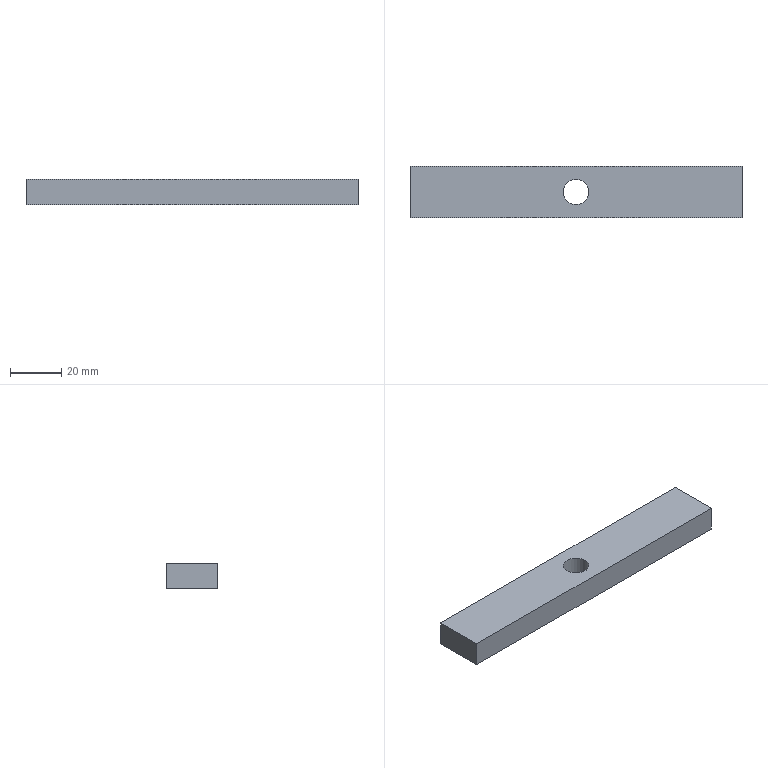Part | NX | features solid 2 | 1 solid | 7 faces | box 130 x 20 x 10 mm | volume 25215 mm3 | plane 6 | cylinder 1 | commonest cylinder face diameters 10 x1
STEP:
#1=CARTESIAN_POINT('',(-65.,437.,-83.));
#2=VERTEX_POINT('',#1);
#3=CARTESIAN_POINT('',(-65.,457.,-83.));
#4=VERTEX_POINT('',#3);
#5=CARTESIAN_POINT('',(-65.,417.,-83.));
#6=DIRECTION('',(0.,1.,0.));
#7=VECTOR('',#6,1000.);
#8=LINE('',#5,#7);
#9=EDGE_CURVE('',#2,#4,#8,.T.);
#10=ORIENTED_EDGE('',*,*,#9,.F.);
#11=CARTESIAN_POINT('',(-65.,437.,-73.));
#12=VERTEX_POINT('',#11);
#13=CARTESIAN_POINT('',(-65.,437.,-73.));
#14=DIRECTION('',(0.,0.,-1.));
#15=VECTOR('',#14,1000.);
#16=LINE('',#13,#15);
#17=EDGE_CURVE('',#12,#2,#16,.T.);
#18=ORIENTED_EDGE('',*,*,#17,.F.);
#19=CARTESIAN_POINT('',(-65.,457.,-73.));
#20=VERTEX_POINT('',#19);
#21=CARTESIAN_POINT('',(-65.,457.,-73.));
#22=DIRECTION('',(0.,-1.,0.));
#23=VECTOR('',#22,1000.);
#24=LINE('',#21,#23);
#25=EDGE_CURVE('',#12,#20,#24,.F.);
#26=ORIENTED_EDGE('',*,*,#25,.T.);
#27=CARTESIAN_POINT('',(-65.,457.,-73.));
#28=DIRECTION('',(0.,0.,-1.));
#29=VECTOR('',#28,1000.);
#30=LINE('',#27,#29);
#31=EDGE_CURVE('',#20,#4,#30,.T.);
#32=ORIENTED_EDGE('',*,*,#31,.T.);
#33=EDGE_LOOP('',(#10,#18,#26,#32));
#34=FACE_BOUND('',#33,.T.);
#35=CARTESIAN_POINT('',(-65.,457.,-73.));
#36=DIRECTION('',(-1.,0.,0.));
#37=DIRECTION('',(0.,0.,-1.));
#38=AXIS2_PLACEMENT_3D('',#35,#36,#37);
#39=PLANE('',#38);
#40=ADVANCED_FACE('',(#34),#39,.T.);
#41=CARTESIAN_POINT('',(-5.,447.,-73.));
#42=VERTEX_POINT('',#41);
#43=CARTESIAN_POINT('',(0.,447.,-73.));
#44=DIRECTION('',(0.,0.,-1.));
#45=DIRECTION('',(-1.,0.,0.));
#46=AXIS2_PLACEMENT_3D('',#43,#44,#45);
#47=CIRCLE('',#46,5.);
#48=EDGE_CURVE('',#42,#42,#47,.F.);
#49=ORIENTED_EDGE('',*,*,#48,.F.);
#50=EDGE_LOOP('',(#49));
#51=FACE_BOUND('',#50,.T.);
#52=ORIENTED_EDGE('',*,*,#25,.F.);
#53=CARTESIAN_POINT('',(65.,437.,-73.));
#54=VERTEX_POINT('',#53);
#55=CARTESIAN_POINT('',(-35.,437.,-73.));
#56=DIRECTION('',(1.,0.,0.));
#57=VECTOR('',#56,1000.);
#58=LINE('',#55,#57);
#59=EDGE_CURVE('',#12,#54,#58,.T.);
#60=ORIENTED_EDGE('',*,*,#59,.T.);
#61=CARTESIAN_POINT('',(65.,457.,-73.));
#62=VERTEX_POINT('',#61);
#63=CARTESIAN_POINT('',(65.,417.,-73.));
#64=DIRECTION('',(0.,1.,0.));
#65=VECTOR('',#64,1000.);
#66=LINE('',#63,#65);
#67=EDGE_CURVE('',#54,#62,#66,.T.);
#68=ORIENTED_EDGE('',*,*,#67,.T.);
#69=CARTESIAN_POINT('',(-35.,457.,-73.));
#70=DIRECTION('',(1.,0.,0.));
#71=VECTOR('',#70,1000.);
#72=LINE('',#69,#71);
#73=EDGE_CURVE('',#20,#62,#72,.T.);
#74=ORIENTED_EDGE('',*,*,#73,.F.);
#75=EDGE_LOOP('',(#52,#60,#68,#74));
#76=FACE_BOUND('',#75,.T.);
#77=CARTESIAN_POINT('',(-35.,417.,-73.));
#78=DIRECTION('',(0.,0.,-1.));
#79=DIRECTION('',(1.,0.,0.));
#80=AXIS2_PLACEMENT_3D('',#77,#78,#79);
#81=PLANE('',#80);
#82=ADVANCED_FACE('',(#51,#76),#81,.F.);
#83=ORIENTED_EDGE('',*,*,#67,.F.);
#84=CARTESIAN_POINT('',(65.,437.,-83.));
#85=VERTEX_POINT('',#84);
#86=CARTESIAN_POINT('',(65.,437.,-73.));
#87=DIRECTION('',(0.,0.,-1.));
#88=VECTOR('',#87,1000.);
#89=LINE('',#86,#88);
#90=EDGE_CURVE('',#54,#85,#89,.T.);
#91=ORIENTED_EDGE('',*,*,#90,.T.);
#92=CARTESIAN_POINT('',(65.,457.,-83.));
#93=VERTEX_POINT('',#92);
#94=CARTESIAN_POINT('',(65.,417.,-83.));
#95=DIRECTION('',(0.,1.,0.));
#96=VECTOR('',#95,1000.);
#97=LINE('',#94,#96);
#98=EDGE_CURVE('',#85,#93,#97,.T.);
#99=ORIENTED_EDGE('',*,*,#98,.T.);
#100=CARTESIAN_POINT('',(65.,457.,-73.));
#101=DIRECTION('',(0.,0.,-1.));
#102=VECTOR('',#101,1000.);
#103=LINE('',#100,#102);
#104=EDGE_CURVE('',#62,#93,#103,.T.);
#105=ORIENTED_EDGE('',*,*,#104,.F.);
#106=EDGE_LOOP('',(#83,#91,#99,#105));
#107=FACE_BOUND('',#106,.T.);
#108=CARTESIAN_POINT('',(65.,417.,-73.));
#109=DIRECTION('',(-1.,0.,0.));
#110=DIRECTION('',(0.,0.,-1.));
#111=AXIS2_PLACEMENT_3D('',#108,#109,#110);
#112=PLANE('',#111);
#113=ADVANCED_FACE('',(#107),#112,.F.);
#114=ORIENTED_EDGE('',*,*,#104,.T.);
#115=CARTESIAN_POINT('',(-35.,457.,-83.));
#116=DIRECTION('',(1.,0.,0.));
#117=VECTOR('',#116,1000.);
#118=LINE('',#115,#117);
#119=EDGE_CURVE('',#4,#93,#118,.T.);
#120=ORIENTED_EDGE('',*,*,#119,.F.);
#121=ORIENTED_EDGE('',*,*,#31,.F.);
#122=ORIENTED_EDGE('',*,*,#73,.T.);
#123=EDGE_LOOP('',(#114,#120,#121,#122));
#124=FACE_BOUND('',#123,.T.);
#125=CARTESIAN_POINT('',(-35.,457.,-73.));
#126=DIRECTION('',(0.,-1.,0.));
#127=DIRECTION('',(0.,0.,-1.));
#128=AXIS2_PLACEMENT_3D('',#125,#126,#127);
#129=PLANE('',#128);
#130=ADVANCED_FACE('',(#124),#129,.F.);
#131=CARTESIAN_POINT('',(-5.,447.,-83.));
#132=VERTEX_POINT('',#131);
#133=CARTESIAN_POINT('',(0.,447.,-83.));
#134=DIRECTION('',(0.,0.,-1.));
#135=DIRECTION('',(-1.,0.,0.));
#136=AXIS2_PLACEMENT_3D('',#133,#134,#135);
#137=CIRCLE('',#136,5.);
#138=EDGE_CURVE('',#132,#132,#137,.T.);
#139=ORIENTED_EDGE('',*,*,#138,.F.);
#140=EDGE_LOOP('',(#139));
#141=FACE_BOUND('',#140,.T.);
#142=CARTESIAN_POINT('',(-35.,437.,-83.));
#143=DIRECTION('',(1.,0.,0.));
#144=VECTOR('',#143,1000.);
#145=LINE('',#142,#144);
#146=EDGE_CURVE('',#2,#85,#145,.T.);
#147=ORIENTED_EDGE('',*,*,#146,.F.);
#148=ORIENTED_EDGE('',*,*,#9,.T.);
#149=ORIENTED_EDGE('',*,*,#119,.T.);
#150=ORIENTED_EDGE('',*,*,#98,.F.);
#151=EDGE_LOOP('',(#147,#148,#149,#150));
#152=FACE_BOUND('',#151,.T.);
#153=CARTESIAN_POINT('',(-35.,417.,-83.));
#154=DIRECTION('',(0.,0.,-1.));
#155=DIRECTION('',(1.,0.,0.));
#156=AXIS2_PLACEMENT_3D('',#153,#154,#155);
#157=PLANE('',#156);
#158=ADVANCED_FACE('',(#141,#152),#157,.T.);
#159=ORIENTED_EDGE('',*,*,#90,.F.);
#160=ORIENTED_EDGE('',*,*,#59,.F.);
#161=ORIENTED_EDGE('',*,*,#17,.T.);
#162=ORIENTED_EDGE('',*,*,#146,.T.);
#163=EDGE_LOOP('',(#159,#160,#161,#162));
#164=FACE_BOUND('',#163,.T.);
#165=CARTESIAN_POINT('',(-35.,437.,-73.));
#166=DIRECTION('',(0.,-1.,0.));
#167=DIRECTION('',(0.,0.,-1.));
#168=AXIS2_PLACEMENT_3D('',#165,#166,#167);
#169=PLANE('',#168);
#170=ADVANCED_FACE('',(#164),#169,.T.);
#171=ORIENTED_EDGE('',*,*,#48,.T.);
#172=EDGE_LOOP('',(#171));
#173=FACE_BOUND('',#172,.T.);
#174=ORIENTED_EDGE('',*,*,#138,.T.);
#175=EDGE_LOOP('',(#174));
#176=FACE_BOUND('',#175,.T.);
#177=CARTESIAN_POINT('',(0.,447.,-83.));
#178=DIRECTION('',(0.,0.,-1.));
#179=DIRECTION('',(-1.,0.,0.));
#180=AXIS2_PLACEMENT_3D('',#177,#178,#179);
#181=CYLINDRICAL_SURFACE('',#180,5.);
#182=ADVANCED_FACE('',(#173,#176),#181,.F.);
#183=CLOSED_SHELL('',(#40,#82,#113,#130,#158,#170,#182));
#184=MANIFOLD_SOLID_BREP('',#183);
#185=(LENGTH_UNIT()NAMED_UNIT(*)SI_UNIT(.MILLI.,.METRE.));
#186=UNCERTAINTY_MEASURE_WITH_UNIT(LENGTH_MEASURE(0.00001),#185,'','');
#187=(NAMED_UNIT(*)PLANE_ANGLE_UNIT()SI_UNIT($,.RADIAN.));
#188=(NAMED_UNIT(*)SI_UNIT($,.STERADIAN.)SOLID_ANGLE_UNIT());
#189=(GEOMETRIC_REPRESENTATION_CONTEXT(3)GLOBAL_UNCERTAINTY_ASSIGNED_CONTEXT((#186))GLOBAL_UNIT_ASSIGNED_CONTEXT((#185,#187,#188))REPRESENTATION_CONTEXT('',''));
#190=ADVANCED_BREP_SHAPE_REPRESENTATION('',(#184),#189);